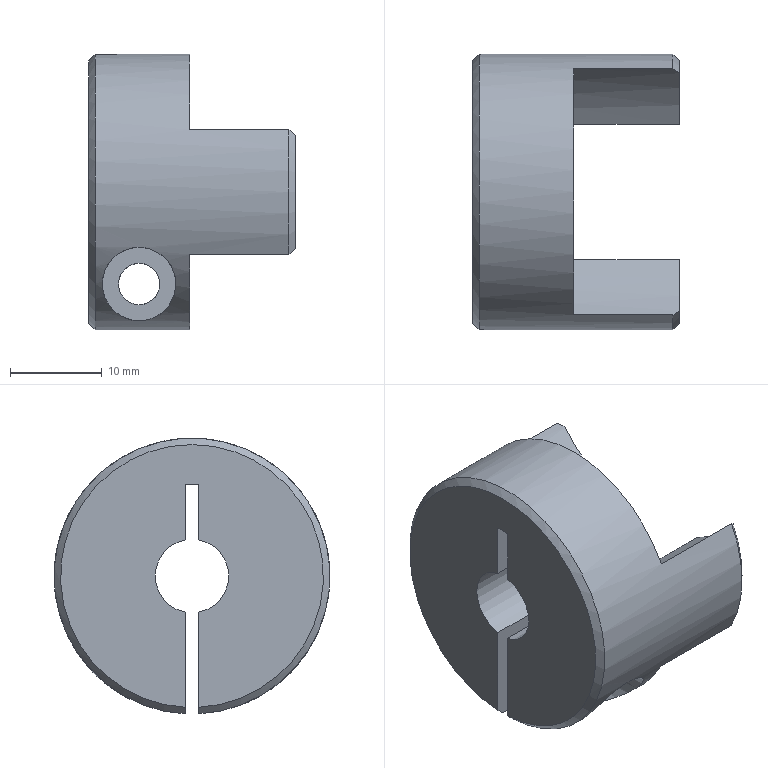Part | NX | features BREP 1 | 1 solid | 28 faces | box 22.5 x 30 x 29.981 mm | volume 7738 mm3 | cylinder 15 | plane 10 | cone 3 | commonest cylinder face diameters 4.5 x4 8 x4 32.5 x4 15 x2 30 x1
STEP:
#1=CARTESIAN_POINT('',(5.5,0.75,-12.25));
#2=VERTEX_POINT('',#1);
#3=CARTESIAN_POINT('',(5.5,0.75,-7.75));
#4=VERTEX_POINT('',#3);
#5=CARTESIAN_POINT('',(5.5,0.75,-10.));
#6=DIRECTION('',(0.,1.,0.));
#7=DIRECTION('',(0.,0.,1.));
#8=AXIS2_PLACEMENT_3D('',#5,#6,#7);
#9=CIRCLE('',#8,2.25);
#10=EDGE_CURVE('',#2,#4,#9,.T.);
#11=ORIENTED_EDGE('',*,*,#10,.F.);
#12=CARTESIAN_POINT('',(5.5,8.657,-12.25));
#13=VERTEX_POINT('',#12);
#14=CARTESIAN_POINT('',(5.5,13.748,-12.25));
#15=DIRECTION('',(0.,1.,0.));
#16=VECTOR('',#15,1000.);
#17=LINE('',#14,#16);
#18=EDGE_CURVE('',#2,#13,#17,.T.);
#19=ORIENTED_EDGE('',*,*,#18,.T.);
#20=CARTESIAN_POINT('',(5.5,12.843,-7.75));
#21=VERTEX_POINT('',#20);
#22=CARTESIAN_POINT('',(5.5,8.657,-12.25));
#23=CARTESIAN_POINT('',(4.786,8.657,-12.25));
#24=CARTESIAN_POINT('',(3.672,9.571,-11.603));
#25=CARTESIAN_POINT('',(3.097,11.052,-10.221));
#26=CARTESIAN_POINT('',(3.478,12.411,-8.494));
#27=CARTESIAN_POINT('',(4.788,12.843,-7.75));
#28=CARTESIAN_POINT('',(5.5,12.843,-7.75));
#29=B_SPLINE_CURVE_WITH_KNOTS('',3,(#22,#23,#24,#25,#26,#27,#28),.UNSPECIFIED.,.F.,.F.,(4,1,1,1,4),(0.,0.002109,0.004218,0.006326,0.008435),.UNSPECIFIED.);
#30=EDGE_CURVE('',#13,#21,#29,.T.);
#31=ORIENTED_EDGE('',*,*,#30,.T.);
#32=CARTESIAN_POINT('',(5.5,13.748,-7.75));
#33=DIRECTION('',(0.,1.,0.));
#34=VECTOR('',#33,1000.);
#35=LINE('',#32,#34);
#36=EDGE_CURVE('',#4,#21,#35,.T.);
#37=ORIENTED_EDGE('',*,*,#36,.F.);
#38=EDGE_LOOP('',(#11,#19,#31,#37));
#39=FACE_BOUND('',#38,.T.);
#40=CARTESIAN_POINT('',(5.5,13.748,-10.));
#41=DIRECTION('',(0.,1.,0.));
#42=DIRECTION('',(0.,0.,-1.));
#43=AXIS2_PLACEMENT_3D('',#40,#41,#42);
#44=CYLINDRICAL_SURFACE('',#43,2.25);
#45=ADVANCED_FACE('',(#39),#44,.F.);
#46=CARTESIAN_POINT('',(5.5,-13.748,-6.));
#47=VERTEX_POINT('',#46);
#48=CARTESIAN_POINT('',(5.5,-5.385,-14.));
#49=VERTEX_POINT('',#48);
#50=CARTESIAN_POINT('',(5.5,-13.748,-6.));
#51=CARTESIAN_POINT('',(4.181,-13.748,-6.));
#52=CARTESIAN_POINT('',(2.328,-13.314,-7.082));
#53=CARTESIAN_POINT('',(1.48,-11.906,-9.196));
#54=CARTESIAN_POINT('',(1.476,-10.6,-10.673));
#55=CARTESIAN_POINT('',(1.92,-9.153,-11.932));
#56=CARTESIAN_POINT('',(2.686,-7.669,-12.929));
#57=CARTESIAN_POINT('',(3.738,-6.207,-13.686));
#58=CARTESIAN_POINT('',(4.838,-5.385,-14.));
#59=CARTESIAN_POINT('',(5.5,-5.385,-14.));
#60=B_SPLINE_CURVE_WITH_KNOTS('',3,(#50,#51,#52,#53,#54,#55,#56,#57,#58,#59),.UNSPECIFIED.,.F.,.F.,(4,1,1,1,1,1,1,4),(0.,0.003899,0.005849,0.007799,0.009748,0.0117,0.01365,0.0156),.UNSPECIFIED.);
#61=EDGE_CURVE('',#47,#49,#60,.T.);
#62=ORIENTED_EDGE('',*,*,#61,.T.);
#63=CARTESIAN_POINT('',(5.5,-4.75,-14.));
#64=VERTEX_POINT('',#63);
#65=CARTESIAN_POINT('',(5.5,13.748,-14.));
#66=DIRECTION('',(0.,1.,0.));
#67=VECTOR('',#66,1000.);
#68=LINE('',#65,#67);
#69=EDGE_CURVE('',#64,#49,#68,.F.);
#70=ORIENTED_EDGE('',*,*,#69,.F.);
#71=CARTESIAN_POINT('',(5.5,-4.75,-6.));
#72=VERTEX_POINT('',#71);
#73=CARTESIAN_POINT('',(5.5,-4.75,-10.));
#74=DIRECTION('',(0.,1.,0.));
#75=DIRECTION('',(0.,0.,1.));
#76=AXIS2_PLACEMENT_3D('',#73,#74,#75);
#77=CIRCLE('',#76,4.);
#78=EDGE_CURVE('',#64,#72,#77,.T.);
#79=ORIENTED_EDGE('',*,*,#78,.T.);
#80=CARTESIAN_POINT('',(5.5,13.748,-6.));
#81=DIRECTION('',(0.,1.,0.));
#82=VECTOR('',#81,1000.);
#83=LINE('',#80,#82);
#84=EDGE_CURVE('',#72,#47,#83,.F.);
#85=ORIENTED_EDGE('',*,*,#84,.T.);
#86=EDGE_LOOP('',(#62,#70,#79,#85));
#87=FACE_BOUND('',#86,.T.);
#88=CARTESIAN_POINT('',(5.5,13.748,-10.));
#89=DIRECTION('',(0.,1.,0.));
#90=DIRECTION('',(0.,0.,-1.));
#91=AXIS2_PLACEMENT_3D('',#88,#89,#90);
#92=CYLINDRICAL_SURFACE('',#91,4.);
#93=ADVANCED_FACE('',(#87),#92,.F.);
#94=CARTESIAN_POINT('',(5.5,-4.75,-12.25));
#95=VERTEX_POINT('',#94);
#96=CARTESIAN_POINT('',(5.5,-4.75,-7.75));
#97=VERTEX_POINT('',#96);
#98=CARTESIAN_POINT('',(5.5,-4.75,-10.));
#99=DIRECTION('',(0.,1.,0.));
#100=DIRECTION('',(0.,0.,1.));
#101=AXIS2_PLACEMENT_3D('',#98,#99,#100);
#102=CIRCLE('',#101,2.25);
#103=EDGE_CURVE('',#95,#97,#102,.T.);
#104=ORIENTED_EDGE('',*,*,#103,.F.);
#105=CARTESIAN_POINT('',(5.5,-0.75,-12.25));
#106=VERTEX_POINT('',#105);
#107=CARTESIAN_POINT('',(5.5,13.748,-12.25));
#108=DIRECTION('',(0.,1.,0.));
#109=VECTOR('',#108,1000.);
#110=LINE('',#107,#109);
#111=EDGE_CURVE('',#95,#106,#110,.T.);
#112=ORIENTED_EDGE('',*,*,#111,.T.);
#113=CARTESIAN_POINT('',(5.5,-0.75,-7.75));
#114=VERTEX_POINT('',#113);
#115=CARTESIAN_POINT('',(5.5,-0.75,-10.));
#116=DIRECTION('',(0.,-1.,0.));
#117=DIRECTION('',(0.,0.,-1.));
#118=AXIS2_PLACEMENT_3D('',#115,#116,#117);
#119=CIRCLE('',#118,2.25);
#120=EDGE_CURVE('',#114,#106,#119,.T.);
#121=ORIENTED_EDGE('',*,*,#120,.F.);
#122=CARTESIAN_POINT('',(5.5,13.748,-7.75));
#123=DIRECTION('',(0.,1.,0.));
#124=VECTOR('',#123,1000.);
#125=LINE('',#122,#124);
#126=EDGE_CURVE('',#97,#114,#125,.T.);
#127=ORIENTED_EDGE('',*,*,#126,.F.);
#128=EDGE_LOOP('',(#104,#112,#121,#127));
#129=FACE_BOUND('',#128,.T.);
#130=CARTESIAN_POINT('',(5.5,13.748,-10.));
#131=DIRECTION('',(0.,1.,0.));
#132=DIRECTION('',(0.,0.,-1.));
#133=AXIS2_PLACEMENT_3D('',#130,#131,#132);
#134=CYLINDRICAL_SURFACE('',#133,2.25);
#135=ADVANCED_FACE('',(#129),#134,.F.);
#136=ORIENTED_EDGE('',*,*,#120,.T.);
#137=CARTESIAN_POINT('',(5.5,-0.75,-10.));
#138=DIRECTION('',(0.,-1.,0.));
#139=DIRECTION('',(0.,0.,-1.));
#140=AXIS2_PLACEMENT_3D('',#137,#138,#139);
#141=CIRCLE('',#140,2.25);
#142=EDGE_CURVE('',#106,#114,#141,.T.);
#143=ORIENTED_EDGE('',*,*,#142,.T.);
#144=EDGE_LOOP('',(#136,#143));
#145=FACE_BOUND('',#144,.T.);
#146=CARTESIAN_POINT('',(0.7071,-0.75,-14.981));
#147=VERTEX_POINT('',#146);
#148=CARTESIAN_POINT('',(11.,-0.75,-14.981));
#149=VERTEX_POINT('',#148);
#150=CARTESIAN_POINT('',(0.,-0.75,-14.981));
#151=DIRECTION('',(1.,0.,0.));
#152=VECTOR('',#151,1000.);
#153=LINE('',#150,#152);
#154=EDGE_CURVE('',#147,#149,#153,.T.);
#155=ORIENTED_EDGE('',*,*,#154,.F.);
#156=CARTESIAN_POINT('',(0.,-0.75,-14.273));
#157=VERTEX_POINT('',#156);
#158=CARTESIAN_POINT('',(0.7071,-0.75,-14.981));
#159=CARTESIAN_POINT('',(0.4714,-0.75,-14.745));
#160=CARTESIAN_POINT('',(0.2357,-0.75,-14.509));
#161=CARTESIAN_POINT('',(0.,-0.75,-14.273));
#162=B_SPLINE_CURVE_WITH_KNOTS('',3,(#158,#159,#160,#161),.UNSPECIFIED.,.F.,.F.,(4,4),(0.,1.),.PIECEWISE_BEZIER_KNOTS.);
#163=EDGE_CURVE('',#147,#157,#162,.T.);
#164=ORIENTED_EDGE('',*,*,#163,.T.);
#165=CARTESIAN_POINT('',(0.,-0.75,-3.929));
#166=VERTEX_POINT('',#165);
#167=CARTESIAN_POINT('',(0.,-0.75,10.));
#168=DIRECTION('',(0.,0.,-1.));
#169=VECTOR('',#168,1000.);
#170=LINE('',#167,#169);
#171=EDGE_CURVE('',#166,#157,#170,.T.);
#172=ORIENTED_EDGE('',*,*,#171,.F.);
#173=CARTESIAN_POINT('',(11.,-0.75,-3.929));
#174=VERTEX_POINT('',#173);
#175=CARTESIAN_POINT('',(0.,-0.75,-3.929));
#176=DIRECTION('',(1.,0.,0.));
#177=VECTOR('',#176,1000.);
#178=LINE('',#175,#177);
#179=EDGE_CURVE('',#166,#174,#178,.T.);
#180=ORIENTED_EDGE('',*,*,#179,.T.);
#181=CARTESIAN_POINT('',(11.,-0.75,10.));
#182=DIRECTION('',(0.,0.,-1.));
#183=VECTOR('',#182,1000.);
#184=LINE('',#181,#183);
#185=EDGE_CURVE('',#174,#149,#184,.T.);
#186=ORIENTED_EDGE('',*,*,#185,.T.);
#187=EDGE_LOOP('',(#155,#164,#172,#180,#186));
#188=FACE_BOUND('',#187,.T.);
#189=CARTESIAN_POINT('',(0.,-0.75,10.));
#190=DIRECTION('',(0.,-1.,0.));
#191=DIRECTION('',(0.,0.,1.));
#192=AXIS2_PLACEMENT_3D('',#189,#190,#191);
#193=PLANE('',#192);
#194=ADVANCED_FACE('',(#145,#188),#193,.F.);
#195=CARTESIAN_POINT('',(0.,0.75,3.929));
#196=VERTEX_POINT('',#195);
#197=CARTESIAN_POINT('',(0.,0.75,10.));
#198=VERTEX_POINT('',#197);
#199=CARTESIAN_POINT('',(0.,0.75,-14.981));
#200=DIRECTION('',(0.,0.,1.));
#201=VECTOR('',#200,1000.);
#202=LINE('',#199,#201);
#203=EDGE_CURVE('',#196,#198,#202,.T.);
#204=ORIENTED_EDGE('',*,*,#203,.F.);
#205=CARTESIAN_POINT('',(11.,0.75,3.929));
#206=VERTEX_POINT('',#205);
#207=CARTESIAN_POINT('',(0.,0.75,3.929));
#208=DIRECTION('',(1.,0.,0.));
#209=VECTOR('',#208,1000.);
#210=LINE('',#207,#209);
#211=EDGE_CURVE('',#196,#206,#210,.T.);
#212=ORIENTED_EDGE('',*,*,#211,.T.);
#213=CARTESIAN_POINT('',(11.,0.75,10.));
#214=VERTEX_POINT('',#213);
#215=CARTESIAN_POINT('',(11.,0.75,-14.981));
#216=DIRECTION('',(0.,0.,1.));
#217=VECTOR('',#216,1000.);
#218=LINE('',#215,#217);
#219=EDGE_CURVE('',#206,#214,#218,.T.);
#220=ORIENTED_EDGE('',*,*,#219,.T.);
#221=CARTESIAN_POINT('',(0.,0.75,10.));
#222=DIRECTION('',(1.,0.,0.));
#223=VECTOR('',#222,1000.);
#224=LINE('',#221,#223);
#225=EDGE_CURVE('',#198,#214,#224,.T.);
#226=ORIENTED_EDGE('',*,*,#225,.F.);
#227=EDGE_LOOP('',(#204,#212,#220,#226));
#228=FACE_BOUND('',#227,.T.);
#229=CARTESIAN_POINT('',(0.,0.75,-14.981));
#230=DIRECTION('',(0.,1.,0.));
#231=DIRECTION('',(0.,0.,-1.));
#232=AXIS2_PLACEMENT_3D('',#229,#230,#231);
#233=PLANE('',#232);
#234=ADVANCED_FACE('',(#228),#233,.F.);
#235=CARTESIAN_POINT('',(11.,-0.75,3.929));
#236=VERTEX_POINT('',#235);
#237=CARTESIAN_POINT('',(11.,0.,0.));
#238=DIRECTION('',(1.,0.,0.));
#239=DIRECTION('',(0.,0.,-1.));
#240=AXIS2_PLACEMENT_3D('',#237,#238,#239);
#241=CIRCLE('',#240,4.);
#242=EDGE_CURVE('',#236,#174,#241,.T.);
#243=ORIENTED_EDGE('',*,*,#242,.F.);
#244=CARTESIAN_POINT('',(11.,-0.75,10.));
#245=VERTEX_POINT('',#244);
#246=CARTESIAN_POINT('',(11.,-0.75,10.));
#247=DIRECTION('',(0.,0.,-1.));
#248=VECTOR('',#247,1000.);
#249=LINE('',#246,#248);
#250=EDGE_CURVE('',#245,#236,#249,.T.);
#251=ORIENTED_EDGE('',*,*,#250,.F.);
#252=CARTESIAN_POINT('',(11.,0.75,10.));
#253=DIRECTION('',(0.,-1.,0.));
#254=VECTOR('',#253,1000.);
#255=LINE('',#252,#254);
#256=EDGE_CURVE('',#214,#245,#255,.T.);
#257=ORIENTED_EDGE('',*,*,#256,.F.);
#258=ORIENTED_EDGE('',*,*,#219,.F.);
#259=CARTESIAN_POINT('',(11.,0.75,-3.929));
#260=VERTEX_POINT('',#259);
#261=CARTESIAN_POINT('',(11.,0.,0.));
#262=DIRECTION('',(1.,0.,0.));
#263=DIRECTION('',(0.,0.,-1.));
#264=AXIS2_PLACEMENT_3D('',#261,#262,#263);
#265=CIRCLE('',#264,4.);
#266=EDGE_CURVE('',#260,#206,#265,.T.);
#267=ORIENTED_EDGE('',*,*,#266,.F.);
#268=CARTESIAN_POINT('',(11.,0.75,-14.981));
#269=VERTEX_POINT('',#268);
#270=CARTESIAN_POINT('',(11.,0.75,-14.981));
#271=DIRECTION('',(0.,0.,1.));
#272=VECTOR('',#271,1000.);
#273=LINE('',#270,#272);
#274=EDGE_CURVE('',#269,#260,#273,.T.);
#275=ORIENTED_EDGE('',*,*,#274,.F.);
#276=CARTESIAN_POINT('',(11.,13.381,-6.779));
#277=VERTEX_POINT('',#276);
#278=CARTESIAN_POINT('',(11.,0.,0.));
#279=DIRECTION('',(1.,0.,0.));
#280=DIRECTION('',(0.,0.,-1.));
#281=AXIS2_PLACEMENT_3D('',#278,#279,#280);
#282=CIRCLE('',#281,15.);
#283=EDGE_CURVE('',#269,#277,#282,.T.);
#284=ORIENTED_EDGE('',*,*,#283,.T.);
#285=CARTESIAN_POINT('',(11.,7.347,-1.506));
#286=VERTEX_POINT('',#285);
#287=CARTESIAN_POINT('',(11.,0.,-16.));
#288=DIRECTION('',(-1.,0.,0.));
#289=DIRECTION('',(0.,0.,-1.));
#290=AXIS2_PLACEMENT_3D('',#287,#288,#289);
#291=CIRCLE('',#290,16.25);
#292=EDGE_CURVE('',#286,#277,#291,.T.);
#293=ORIENTED_EDGE('',*,*,#292,.F.);
#294=CARTESIAN_POINT('',(11.,7.347,1.506));
#295=VERTEX_POINT('',#294);
#296=CARTESIAN_POINT('',(11.,0.,0.));
#297=DIRECTION('',(-1.,0.,0.));
#298=DIRECTION('',(0.,0.,-1.));
#299=AXIS2_PLACEMENT_3D('',#296,#297,#298);
#300=CIRCLE('',#299,7.5);
#301=EDGE_CURVE('',#295,#286,#300,.T.);
#302=ORIENTED_EDGE('',*,*,#301,.F.);
#303=CARTESIAN_POINT('',(11.,13.381,6.779));
#304=VERTEX_POINT('',#303);
#305=CARTESIAN_POINT('',(11.,0.,16.));
#306=DIRECTION('',(-1.,0.,0.));
#307=DIRECTION('',(0.,0.,-1.));
#308=AXIS2_PLACEMENT_3D('',#305,#306,#307);
#309=CIRCLE('',#308,16.25);
#310=EDGE_CURVE('',#304,#295,#309,.T.);
#311=ORIENTED_EDGE('',*,*,#310,.F.);
#312=CARTESIAN_POINT('',(11.,-13.381,6.779));
#313=VERTEX_POINT('',#312);
#314=CARTESIAN_POINT('',(11.,0.,0.));
#315=DIRECTION('',(1.,0.,0.));
#316=DIRECTION('',(0.,0.,-1.));
#317=AXIS2_PLACEMENT_3D('',#314,#315,#316);
#318=CIRCLE('',#317,15.);
#319=EDGE_CURVE('',#304,#313,#318,.T.);
#320=ORIENTED_EDGE('',*,*,#319,.T.);
#321=CARTESIAN_POINT('',(11.,-7.347,1.506));
#322=VERTEX_POINT('',#321);
#323=CARTESIAN_POINT('',(11.,0.,16.));
#324=DIRECTION('',(1.,0.,0.));
#325=DIRECTION('',(0.,0.,-1.));
#326=AXIS2_PLACEMENT_3D('',#323,#324,#325);
#327=CIRCLE('',#326,16.25);
#328=EDGE_CURVE('',#313,#322,#327,.T.);
#329=ORIENTED_EDGE('',*,*,#328,.T.);
#330=CARTESIAN_POINT('',(11.,-7.347,-1.506));
#331=VERTEX_POINT('',#330);
#332=CARTESIAN_POINT('',(11.,0.,0.));
#333=DIRECTION('',(1.,0.,0.));
#334=DIRECTION('',(0.,0.,-1.));
#335=AXIS2_PLACEMENT_3D('',#332,#333,#334);
#336=CIRCLE('',#335,7.5);
#337=EDGE_CURVE('',#322,#331,#336,.T.);
#338=ORIENTED_EDGE('',*,*,#337,.T.);
#339=CARTESIAN_POINT('',(11.,-13.381,-6.779));
#340=VERTEX_POINT('',#339);
#341=CARTESIAN_POINT('',(11.,0.,-16.));
#342=DIRECTION('',(1.,0.,0.));
#343=DIRECTION('',(0.,0.,-1.));
#344=AXIS2_PLACEMENT_3D('',#341,#342,#343);
#345=CIRCLE('',#344,16.25);
#346=EDGE_CURVE('',#331,#340,#345,.T.);
#347=ORIENTED_EDGE('',*,*,#346,.T.);
#348=CARTESIAN_POINT('',(11.,0.,0.));
#349=DIRECTION('',(1.,0.,0.));
#350=DIRECTION('',(0.,0.,-1.));
#351=AXIS2_PLACEMENT_3D('',#348,#349,#350);
#352=CIRCLE('',#351,15.);
#353=EDGE_CURVE('',#340,#149,#352,.T.);
#354=ORIENTED_EDGE('',*,*,#353,.T.);
#355=ORIENTED_EDGE('',*,*,#185,.F.);
#356=EDGE_LOOP('',(#243,#251,#257,#258,#267,#275,#284,#293,#302,#311,#320,#329,#338,#347,#354,#355));
#357=FACE_BOUND('',#356,.T.);
#358=CARTESIAN_POINT('',(11.,0.,8.));
#359=DIRECTION('',(1.,0.,0.));
#360=DIRECTION('',(0.,0.,1.));
#361=AXIS2_PLACEMENT_3D('',#358,#359,#360);
#362=PLANE('',#361);
#363=ADVANCED_FACE('',(#357),#362,.T.);
#364=CARTESIAN_POINT('',(5.5,12.843,-7.75));
#365=CARTESIAN_POINT('',(6.211,12.843,-7.75));
#366=CARTESIAN_POINT('',(7.521,12.413,-8.492));
#367=CARTESIAN_POINT('',(7.904,11.052,-10.221));
#368=CARTESIAN_POINT('',(7.328,9.571,-11.603));
#369=CARTESIAN_POINT('',(6.214,8.657,-12.25));
#370=CARTESIAN_POINT('',(5.5,8.657,-12.25));
#371=B_SPLINE_CURVE_WITH_KNOTS('',3,(#364,#365,#366,#367,#368,#369,#370),.UNSPECIFIED.,.F.,.F.,(4,1,1,1,4),(0.,0.0021,0.004201,0.006301,0.008402),.UNSPECIFIED.);
#372=EDGE_CURVE('',#21,#13,#371,.T.);
#373=ORIENTED_EDGE('',*,*,#372,.F.);
#374=ORIENTED_EDGE('',*,*,#30,.F.);
#375=EDGE_LOOP('',(#373,#374));
#376=FACE_BOUND('',#375,.T.);
#377=ORIENTED_EDGE('',*,*,#61,.F.);
#378=CARTESIAN_POINT('',(5.5,-5.385,-14.));
#379=CARTESIAN_POINT('',(6.165,-5.385,-14.));
#380=CARTESIAN_POINT('',(7.265,-6.212,-13.683));
#381=CARTESIAN_POINT('',(8.31,-7.662,-12.934));
#382=CARTESIAN_POINT('',(9.083,-9.162,-11.923));
#383=CARTESIAN_POINT('',(9.667,-11.064,-10.283));
#384=CARTESIAN_POINT('',(9.299,-13.162,-7.484));
#385=CARTESIAN_POINT('',(6.823,-13.748,-6.));
#386=CARTESIAN_POINT('',(5.5,-13.748,-6.));
#387=B_SPLINE_CURVE_WITH_KNOTS('',3,(#378,#379,#380,#381,#382,#383,#384,#385,#386),.UNSPECIFIED.,.F.,.F.,(4,1,1,1,1,1,4),(0.,0.001957,0.003915,0.005872,0.00783,0.01174,0.01566),.UNSPECIFIED.);
#388=EDGE_CURVE('',#49,#47,#387,.T.);
#389=ORIENTED_EDGE('',*,*,#388,.F.);
#390=EDGE_LOOP('',(#377,#389));
#391=FACE_BOUND('',#390,.T.);
#392=CARTESIAN_POINT('',(21.793,-13.381,-6.779));
#393=VERTEX_POINT('',#392);
#394=CARTESIAN_POINT('',(11.,-13.381,-6.779));
#395=DIRECTION('',(1.,0.,0.));
#396=VECTOR('',#395,1000.);
#397=LINE('',#394,#396);
#398=EDGE_CURVE('',#340,#393,#397,.T.);
#399=ORIENTED_EDGE('',*,*,#398,.T.);
#400=CARTESIAN_POINT('',(21.793,-13.381,6.779));
#401=VERTEX_POINT('',#400);
#402=CARTESIAN_POINT('',(21.793,0.,0.));
#403=DIRECTION('',(-1.,0.,0.));
#404=DIRECTION('',(0.,0.,-1.));
#405=AXIS2_PLACEMENT_3D('',#402,#403,#404);
#406=CIRCLE('',#405,15.);
#407=EDGE_CURVE('',#393,#401,#406,.T.);
#408=ORIENTED_EDGE('',*,*,#407,.T.);
#409=CARTESIAN_POINT('',(11.,-13.381,6.779));
#410=DIRECTION('',(1.,0.,0.));
#411=VECTOR('',#410,1000.);
#412=LINE('',#409,#411);
#413=EDGE_CURVE('',#313,#401,#412,.T.);
#414=ORIENTED_EDGE('',*,*,#413,.F.);
#415=ORIENTED_EDGE('',*,*,#319,.F.);
#416=CARTESIAN_POINT('',(21.793,13.381,6.779));
#417=VERTEX_POINT('',#416);
#418=CARTESIAN_POINT('',(22.5,13.381,6.779));
#419=DIRECTION('',(-1.,0.,0.));
#420=VECTOR('',#419,1000.);
#421=LINE('',#418,#420);
#422=EDGE_CURVE('',#417,#304,#421,.T.);
#423=ORIENTED_EDGE('',*,*,#422,.F.);
#424=CARTESIAN_POINT('',(21.793,13.381,-6.779));
#425=VERTEX_POINT('',#424);
#426=CARTESIAN_POINT('',(21.793,0.,0.));
#427=DIRECTION('',(-1.,0.,0.));
#428=DIRECTION('',(0.,0.,-1.));
#429=AXIS2_PLACEMENT_3D('',#426,#427,#428);
#430=CIRCLE('',#429,15.);
#431=EDGE_CURVE('',#417,#425,#430,.T.);
#432=ORIENTED_EDGE('',*,*,#431,.T.);
#433=CARTESIAN_POINT('',(22.5,13.381,-6.779));
#434=DIRECTION('',(-1.,0.,0.));
#435=VECTOR('',#434,1000.);
#436=LINE('',#433,#435);
#437=EDGE_CURVE('',#425,#277,#436,.T.);
#438=ORIENTED_EDGE('',*,*,#437,.T.);
#439=ORIENTED_EDGE('',*,*,#283,.F.);
#440=CARTESIAN_POINT('',(0.7071,0.75,-14.981));
#441=VERTEX_POINT('',#440);
#442=CARTESIAN_POINT('',(0.,0.75,-14.981));
#443=DIRECTION('',(1.,0.,0.));
#444=VECTOR('',#443,1000.);
#445=LINE('',#442,#444);
#446=EDGE_CURVE('',#441,#269,#445,.T.);
#447=ORIENTED_EDGE('',*,*,#446,.F.);
#448=CARTESIAN_POINT('',(0.7071,0.,0.));
#449=DIRECTION('',(1.,0.,0.));
#450=DIRECTION('',(0.,0.,1.));
#451=AXIS2_PLACEMENT_3D('',#448,#449,#450);
#452=CIRCLE('',#451,15.);
#453=EDGE_CURVE('',#441,#147,#452,.T.);
#454=ORIENTED_EDGE('',*,*,#453,.T.);
#455=ORIENTED_EDGE('',*,*,#154,.T.);
#456=ORIENTED_EDGE('',*,*,#353,.F.);
#457=EDGE_LOOP('',(#399,#408,#414,#415,#423,#432,#438,#439,#447,#454,#455,#456));
#458=FACE_BOUND('',#457,.T.);
#459=CARTESIAN_POINT('',(0.,0.,0.));
#460=DIRECTION('',(1.,0.,0.));
#461=DIRECTION('',(0.,0.,1.));
#462=AXIS2_PLACEMENT_3D('',#459,#460,#461);
#463=CYLINDRICAL_SURFACE('',#462,15.);
#464=ADVANCED_FACE('',(#376,#391,#458),#463,.T.);
#465=ORIENTED_EDGE('',*,*,#171,.T.);
#466=CARTESIAN_POINT('',(0.,0.75,-14.273));
#467=VERTEX_POINT('',#466);
#468=CARTESIAN_POINT('',(0.,0.,0.));
#469=DIRECTION('',(-1.,0.,0.));
#470=DIRECTION('',(0.,0.,1.));
#471=AXIS2_PLACEMENT_3D('',#468,#469,#470);
#472=CIRCLE('',#471,14.293);
#473=EDGE_CURVE('',#157,#467,#472,.T.);
#474=ORIENTED_EDGE('',*,*,#473,.T.);
#475=CARTESIAN_POINT('',(0.,0.75,-3.929));
#476=VERTEX_POINT('',#475);
#477=CARTESIAN_POINT('',(0.,0.75,-14.981));
#478=DIRECTION('',(0.,0.,1.));
#479=VECTOR('',#478,1000.);
#480=LINE('',#477,#479);
#481=EDGE_CURVE('',#467,#476,#480,.T.);
#482=ORIENTED_EDGE('',*,*,#481,.T.);
#483=CARTESIAN_POINT('',(0.,0.,0.));
#484=DIRECTION('',(1.,0.,0.));
#485=DIRECTION('',(0.,0.,-1.));
#486=AXIS2_PLACEMENT_3D('',#483,#484,#485);
#487=CIRCLE('',#486,4.);
#488=EDGE_CURVE('',#476,#196,#487,.T.);
#489=ORIENTED_EDGE('',*,*,#488,.T.);
#490=ORIENTED_EDGE('',*,*,#203,.T.);
#491=CARTESIAN_POINT('',(0.,-0.75,10.));
#492=VERTEX_POINT('',#491);
#493=CARTESIAN_POINT('',(0.,0.75,10.));
#494=DIRECTION('',(0.,-1.,0.));
#495=VECTOR('',#494,1000.);
#496=LINE('',#493,#495);
#497=EDGE_CURVE('',#198,#492,#496,.T.);
#498=ORIENTED_EDGE('',*,*,#497,.T.);
#499=CARTESIAN_POINT('',(0.,-0.75,3.929));
#500=VERTEX_POINT('',#499);
#501=CARTESIAN_POINT('',(0.,-0.75,10.));
#502=DIRECTION('',(0.,0.,-1.));
#503=VECTOR('',#502,1000.);
#504=LINE('',#501,#503);
#505=EDGE_CURVE('',#492,#500,#504,.T.);
#506=ORIENTED_EDGE('',*,*,#505,.T.);
#507=CARTESIAN_POINT('',(0.,0.,0.));
#508=DIRECTION('',(1.,0.,0.));
#509=DIRECTION('',(0.,0.,-1.));
#510=AXIS2_PLACEMENT_3D('',#507,#508,#509);
#511=CIRCLE('',#510,4.);
#512=EDGE_CURVE('',#500,#166,#511,.T.);
#513=ORIENTED_EDGE('',*,*,#512,.T.);
#514=EDGE_LOOP('',(#465,#474,#482,#489,#490,#498,#506,#513));
#515=FACE_BOUND('',#514,.T.);
#516=CARTESIAN_POINT('',(0.,15.,0.));
#517=DIRECTION('',(-1.,0.,0.));
#518=DIRECTION('',(0.,0.,-1.));
#519=AXIS2_PLACEMENT_3D('',#516,#517,#518);
#520=PLANE('',#519);
#521=ADVANCED_FACE('',(#515),#520,.T.);
#522=CARTESIAN_POINT('',(22.5,-12.911,6.132));
#523=VERTEX_POINT('',#522);
#524=CARTESIAN_POINT('',(22.5,-7.347,1.506));
#525=VERTEX_POINT('',#524);
#526=CARTESIAN_POINT('',(22.5,0.,16.));
#527=DIRECTION('',(1.,0.,0.));
#528=DIRECTION('',(0.,0.,-1.));
#529=AXIS2_PLACEMENT_3D('',#526,#527,#528);
#530=CIRCLE('',#529,16.25);
#531=EDGE_CURVE('',#523,#525,#530,.T.);
#532=ORIENTED_EDGE('',*,*,#531,.F.);
#533=CARTESIAN_POINT('',(22.5,-12.911,-6.132));
#534=VERTEX_POINT('',#533);
#535=CARTESIAN_POINT('',(22.5,0.,0.));
#536=DIRECTION('',(1.,0.,0.));
#537=DIRECTION('',(0.,0.,-1.));
#538=AXIS2_PLACEMENT_3D('',#535,#536,#537);
#539=CIRCLE('',#538,14.293);
#540=EDGE_CURVE('',#523,#534,#539,.T.);
#541=ORIENTED_EDGE('',*,*,#540,.T.);
#542=CARTESIAN_POINT('',(22.5,-7.347,-1.506));
#543=VERTEX_POINT('',#542);
#544=CARTESIAN_POINT('',(22.5,0.,-16.));
#545=DIRECTION('',(1.,0.,0.));
#546=DIRECTION('',(0.,0.,-1.));
#547=AXIS2_PLACEMENT_3D('',#544,#545,#546);
#548=CIRCLE('',#547,16.25);
#549=EDGE_CURVE('',#543,#534,#548,.T.);
#550=ORIENTED_EDGE('',*,*,#549,.F.);
#551=CARTESIAN_POINT('',(22.5,0.,0.));
#552=DIRECTION('',(1.,0.,0.));
#553=DIRECTION('',(0.,0.,-1.));
#554=AXIS2_PLACEMENT_3D('',#551,#552,#553);
#555=CIRCLE('',#554,7.5);
#556=EDGE_CURVE('',#525,#543,#555,.T.);
#557=ORIENTED_EDGE('',*,*,#556,.F.);
#558=EDGE_LOOP('',(#532,#541,#550,#557));
#559=FACE_BOUND('',#558,.T.);
#560=CARTESIAN_POINT('',(22.5,0.,0.));
#561=DIRECTION('',(1.,0.,0.));
#562=DIRECTION('',(0.,0.,1.));
#563=AXIS2_PLACEMENT_3D('',#560,#561,#562);
#564=PLANE('',#563);
#565=ADVANCED_FACE('',(#559),#564,.T.);
#566=ORIENTED_EDGE('',*,*,#549,.T.);
#567=CARTESIAN_POINT('',(22.5,-12.911,-6.132));
#568=CARTESIAN_POINT('',(22.263,-13.072,-6.343));
#569=CARTESIAN_POINT('',(22.028,-13.229,-6.559));
#570=CARTESIAN_POINT('',(21.793,-13.381,-6.779));
#571=B_SPLINE_CURVE_WITH_KNOTS('',3,(#567,#568,#569,#570),.UNSPECIFIED.,.F.,.F.,(4,4),(0.,1.),.PIECEWISE_BEZIER_KNOTS.);
#572=EDGE_CURVE('',#534,#393,#571,.T.);
#573=ORIENTED_EDGE('',*,*,#572,.T.);
#574=ORIENTED_EDGE('',*,*,#398,.F.);
#575=ORIENTED_EDGE('',*,*,#346,.F.);
#576=CARTESIAN_POINT('',(11.,-7.347,-1.506));
#577=DIRECTION('',(1.,0.,0.));
#578=VECTOR('',#577,1000.);
#579=LINE('',#576,#578);
#580=EDGE_CURVE('',#331,#543,#579,.T.);
#581=ORIENTED_EDGE('',*,*,#580,.T.);
#582=EDGE_LOOP('',(#566,#573,#574,#575,#581));
#583=FACE_BOUND('',#582,.T.);
#584=CARTESIAN_POINT('',(11.,0.,-16.));
#585=DIRECTION('',(1.,0.,0.));
#586=DIRECTION('',(0.,0.,1.));
#587=AXIS2_PLACEMENT_3D('',#584,#585,#586);
#588=CYLINDRICAL_SURFACE('',#587,16.25);
#589=ADVANCED_FACE('',(#583),#588,.F.);
#590=ORIENTED_EDGE('',*,*,#556,.T.);
#591=ORIENTED_EDGE('',*,*,#580,.F.);
#592=ORIENTED_EDGE('',*,*,#337,.F.);
#593=CARTESIAN_POINT('',(11.,-7.347,1.506));
#594=DIRECTION('',(1.,0.,0.));
#595=VECTOR('',#594,1000.);
#596=LINE('',#593,#595);
#597=EDGE_CURVE('',#322,#525,#596,.T.);
#598=ORIENTED_EDGE('',*,*,#597,.T.);
#599=EDGE_LOOP('',(#590,#591,#592,#598));
#600=FACE_BOUND('',#599,.T.);
#601=CARTESIAN_POINT('',(11.,0.,0.));
#602=DIRECTION('',(1.,0.,0.));
#603=DIRECTION('',(0.,0.,1.));
#604=AXIS2_PLACEMENT_3D('',#601,#602,#603);
#605=CYLINDRICAL_SURFACE('',#604,7.5);
#606=ADVANCED_FACE('',(#600),#605,.F.);
#607=ORIENTED_EDGE('',*,*,#413,.T.);
#608=CARTESIAN_POINT('',(21.793,-13.381,6.779));
#609=CARTESIAN_POINT('',(22.028,-13.229,6.559));
#610=CARTESIAN_POINT('',(22.263,-13.072,6.343));
#611=CARTESIAN_POINT('',(22.5,-12.911,6.132));
#612=B_SPLINE_CURVE_WITH_KNOTS('',3,(#608,#609,#610,#611),.UNSPECIFIED.,.F.,.F.,(4,4),(0.,1.),.PIECEWISE_BEZIER_KNOTS.);
#613=EDGE_CURVE('',#401,#523,#612,.T.);
#614=ORIENTED_EDGE('',*,*,#613,.T.);
#615=ORIENTED_EDGE('',*,*,#531,.T.);
#616=ORIENTED_EDGE('',*,*,#597,.F.);
#617=ORIENTED_EDGE('',*,*,#328,.F.);
#618=EDGE_LOOP('',(#607,#614,#615,#616,#617));
#619=FACE_BOUND('',#618,.T.);
#620=CARTESIAN_POINT('',(11.,0.,16.));
#621=DIRECTION('',(1.,0.,0.));
#622=DIRECTION('',(0.,0.,1.));
#623=AXIS2_PLACEMENT_3D('',#620,#621,#622);
#624=CYLINDRICAL_SURFACE('',#623,16.25);
#625=ADVANCED_FACE('',(#619),#624,.F.);
#626=ORIENTED_EDGE('',*,*,#250,.T.);
#627=CARTESIAN_POINT('',(0.,-0.75,3.929));
#628=DIRECTION('',(1.,0.,0.));
#629=VECTOR('',#628,1000.);
#630=LINE('',#627,#629);
#631=EDGE_CURVE('',#500,#236,#630,.T.);
#632=ORIENTED_EDGE('',*,*,#631,.F.);
#633=ORIENTED_EDGE('',*,*,#505,.F.);
#634=CARTESIAN_POINT('',(0.,-0.75,10.));
#635=DIRECTION('',(1.,0.,0.));
#636=VECTOR('',#635,1000.);
#637=LINE('',#634,#636);
#638=EDGE_CURVE('',#492,#245,#637,.T.);
#639=ORIENTED_EDGE('',*,*,#638,.T.);
#640=EDGE_LOOP('',(#626,#632,#633,#639));
#641=FACE_BOUND('',#640,.T.);
#642=CARTESIAN_POINT('',(0.,-0.75,10.));
#643=DIRECTION('',(0.,-1.,0.));
#644=DIRECTION('',(0.,0.,1.));
#645=AXIS2_PLACEMENT_3D('',#642,#643,#644);
#646=PLANE('',#645);
#647=ADVANCED_FACE('',(#641),#646,.F.);
#648=ORIENTED_EDGE('',*,*,#256,.T.);
#649=ORIENTED_EDGE('',*,*,#638,.F.);
#650=ORIENTED_EDGE('',*,*,#497,.F.);
#651=ORIENTED_EDGE('',*,*,#225,.T.);
#652=EDGE_LOOP('',(#648,#649,#650,#651));
#653=FACE_BOUND('',#652,.T.);
#654=CARTESIAN_POINT('',(0.,0.75,10.));
#655=DIRECTION('',(0.,0.,1.));
#656=DIRECTION('',(-1.,0.,0.));
#657=AXIS2_PLACEMENT_3D('',#654,#655,#656);
#658=PLANE('',#657);
#659=ADVANCED_FACE('',(#653),#658,.F.);
#660=CARTESIAN_POINT('',(5.5,0.75,-10.));
#661=DIRECTION('',(0.,1.,0.));
#662=DIRECTION('',(0.,0.,1.));
#663=AXIS2_PLACEMENT_3D('',#660,#661,#662);
#664=CIRCLE('',#663,2.25);
#665=EDGE_CURVE('',#4,#2,#664,.T.);
#666=ORIENTED_EDGE('',*,*,#665,.T.);
#667=ORIENTED_EDGE('',*,*,#10,.T.);
#668=EDGE_LOOP('',(#666,#667));
#669=FACE_BOUND('',#668,.T.);
#670=ORIENTED_EDGE('',*,*,#481,.F.);
#671=CARTESIAN_POINT('',(0.,0.75,-14.273));
#672=CARTESIAN_POINT('',(0.2357,0.75,-14.509));
#673=CARTESIAN_POINT('',(0.4714,0.75,-14.745));
#674=CARTESIAN_POINT('',(0.7071,0.75,-14.981));
#675=B_SPLINE_CURVE_WITH_KNOTS('',3,(#671,#672,#673,#674),.UNSPECIFIED.,.F.,.F.,(4,4),(0.,1.),.PIECEWISE_BEZIER_KNOTS.);
#676=EDGE_CURVE('',#467,#441,#675,.T.);
#677=ORIENTED_EDGE('',*,*,#676,.T.);
#678=ORIENTED_EDGE('',*,*,#446,.T.);
#679=ORIENTED_EDGE('',*,*,#274,.T.);
#680=CARTESIAN_POINT('',(0.,0.75,-3.929));
#681=DIRECTION('',(1.,0.,0.));
#682=VECTOR('',#681,1000.);
#683=LINE('',#680,#682);
#684=EDGE_CURVE('',#476,#260,#683,.T.);
#685=ORIENTED_EDGE('',*,*,#684,.F.);
#686=EDGE_LOOP('',(#670,#677,#678,#679,#685));
#687=FACE_BOUND('',#686,.T.);
#688=CARTESIAN_POINT('',(0.,0.75,-14.981));
#689=DIRECTION('',(0.,1.,0.));
#690=DIRECTION('',(0.,0.,-1.));
#691=AXIS2_PLACEMENT_3D('',#688,#689,#690);
#692=PLANE('',#691);
#693=ADVANCED_FACE('',(#669,#687),#692,.F.);
#694=ORIENTED_EDGE('',*,*,#437,.F.);
#695=CARTESIAN_POINT('',(22.5,12.911,-6.132));
#696=VERTEX_POINT('',#695);
#697=CARTESIAN_POINT('',(21.793,13.381,-6.779));
#698=CARTESIAN_POINT('',(22.028,13.229,-6.559));
#699=CARTESIAN_POINT('',(22.263,13.072,-6.343));
#700=CARTESIAN_POINT('',(22.5,12.911,-6.132));
#701=B_SPLINE_CURVE_WITH_KNOTS('',3,(#697,#698,#699,#700),.UNSPECIFIED.,.F.,.F.,(4,4),(0.,1.),.PIECEWISE_BEZIER_KNOTS.);
#702=EDGE_CURVE('',#425,#696,#701,.T.);
#703=ORIENTED_EDGE('',*,*,#702,.T.);
#704=CARTESIAN_POINT('',(22.5,7.347,-1.506));
#705=VERTEX_POINT('',#704);
#706=CARTESIAN_POINT('',(22.5,0.,-16.));
#707=DIRECTION('',(-1.,0.,0.));
#708=DIRECTION('',(0.,0.,-1.));
#709=AXIS2_PLACEMENT_3D('',#706,#707,#708);
#710=CIRCLE('',#709,16.25);
#711=EDGE_CURVE('',#705,#696,#710,.T.);
#712=ORIENTED_EDGE('',*,*,#711,.F.);
#713=CARTESIAN_POINT('',(22.5,7.347,-1.506));
#714=DIRECTION('',(-1.,0.,0.));
#715=VECTOR('',#714,1000.);
#716=LINE('',#713,#715);
#717=EDGE_CURVE('',#705,#286,#716,.T.);
#718=ORIENTED_EDGE('',*,*,#717,.T.);
#719=ORIENTED_EDGE('',*,*,#292,.T.);
#720=EDGE_LOOP('',(#694,#703,#712,#718,#719));
#721=FACE_BOUND('',#720,.T.);
#722=CARTESIAN_POINT('',(22.5,0.,-16.));
#723=DIRECTION('',(-1.,0.,0.));
#724=DIRECTION('',(0.,0.,-1.));
#725=AXIS2_PLACEMENT_3D('',#722,#723,#724);
#726=CYLINDRICAL_SURFACE('',#725,16.25);
#727=ADVANCED_FACE('',(#721),#726,.F.);
#728=CARTESIAN_POINT('',(22.5,12.911,6.132));
#729=VERTEX_POINT('',#728);
#730=CARTESIAN_POINT('',(22.5,7.347,1.506));
#731=VERTEX_POINT('',#730);
#732=CARTESIAN_POINT('',(22.5,0.,16.));
#733=DIRECTION('',(-1.,0.,0.));
#734=DIRECTION('',(0.,0.,-1.));
#735=AXIS2_PLACEMENT_3D('',#732,#733,#734);
#736=CIRCLE('',#735,16.25);
#737=EDGE_CURVE('',#729,#731,#736,.T.);
#738=ORIENTED_EDGE('',*,*,#737,.F.);
#739=CARTESIAN_POINT('',(22.5,12.911,6.132));
#740=CARTESIAN_POINT('',(22.263,13.072,6.343));
#741=CARTESIAN_POINT('',(22.028,13.229,6.559));
#742=CARTESIAN_POINT('',(21.793,13.381,6.779));
#743=B_SPLINE_CURVE_WITH_KNOTS('',3,(#739,#740,#741,#742),.UNSPECIFIED.,.F.,.F.,(4,4),(0.,1.),.PIECEWISE_BEZIER_KNOTS.);
#744=EDGE_CURVE('',#729,#417,#743,.T.);
#745=ORIENTED_EDGE('',*,*,#744,.T.);
#746=ORIENTED_EDGE('',*,*,#422,.T.);
#747=ORIENTED_EDGE('',*,*,#310,.T.);
#748=CARTESIAN_POINT('',(22.5,7.347,1.506));
#749=DIRECTION('',(-1.,0.,0.));
#750=VECTOR('',#749,1000.);
#751=LINE('',#748,#750);
#752=EDGE_CURVE('',#731,#295,#751,.T.);
#753=ORIENTED_EDGE('',*,*,#752,.F.);
#754=EDGE_LOOP('',(#738,#745,#746,#747,#753));
#755=FACE_BOUND('',#754,.T.);
#756=CARTESIAN_POINT('',(22.5,0.,16.));
#757=DIRECTION('',(-1.,0.,0.));
#758=DIRECTION('',(0.,0.,-1.));
#759=AXIS2_PLACEMENT_3D('',#756,#757,#758);
#760=CYLINDRICAL_SURFACE('',#759,16.25);
#761=ADVANCED_FACE('',(#755),#760,.F.);
#762=ORIENTED_EDGE('',*,*,#301,.T.);
#763=ORIENTED_EDGE('',*,*,#717,.F.);
#764=CARTESIAN_POINT('',(22.5,0.,0.));
#765=DIRECTION('',(-1.,0.,0.));
#766=DIRECTION('',(0.,0.,-1.));
#767=AXIS2_PLACEMENT_3D('',#764,#765,#766);
#768=CIRCLE('',#767,7.5);
#769=EDGE_CURVE('',#731,#705,#768,.T.);
#770=ORIENTED_EDGE('',*,*,#769,.F.);
#771=ORIENTED_EDGE('',*,*,#752,.T.);
#772=EDGE_LOOP('',(#762,#763,#770,#771));
#773=FACE_BOUND('',#772,.T.);
#774=CARTESIAN_POINT('',(22.5,0.,0.));
#775=DIRECTION('',(-1.,0.,0.));
#776=DIRECTION('',(0.,0.,-1.));
#777=AXIS2_PLACEMENT_3D('',#774,#775,#776);
#778=CYLINDRICAL_SURFACE('',#777,7.5);
#779=ADVANCED_FACE('',(#773),#778,.F.);
#780=ORIENTED_EDGE('',*,*,#711,.T.);
#781=CARTESIAN_POINT('',(22.5,0.,0.));
#782=DIRECTION('',(1.,0.,0.));
#783=DIRECTION('',(0.,0.,-1.));
#784=AXIS2_PLACEMENT_3D('',#781,#782,#783);
#785=CIRCLE('',#784,14.293);
#786=EDGE_CURVE('',#696,#729,#785,.T.);
#787=ORIENTED_EDGE('',*,*,#786,.T.);
#788=ORIENTED_EDGE('',*,*,#737,.T.);
#789=ORIENTED_EDGE('',*,*,#769,.T.);
#790=EDGE_LOOP('',(#780,#787,#788,#789));
#791=FACE_BOUND('',#790,.T.);
#792=CARTESIAN_POINT('',(22.5,0.,-8.));
#793=DIRECTION('',(1.,0.,0.));
#794=DIRECTION('',(0.,0.,1.));
#795=AXIS2_PLACEMENT_3D('',#792,#793,#794);
#796=PLANE('',#795);
#797=ADVANCED_FACE('',(#791),#796,.T.);
#798=ORIENTED_EDGE('',*,*,#266,.T.);
#799=ORIENTED_EDGE('',*,*,#211,.F.);
#800=ORIENTED_EDGE('',*,*,#488,.F.);
#801=ORIENTED_EDGE('',*,*,#684,.T.);
#802=EDGE_LOOP('',(#798,#799,#800,#801));
#803=FACE_BOUND('',#802,.T.);
#804=CARTESIAN_POINT('',(0.,0.,0.));
#805=DIRECTION('',(1.,0.,0.));
#806=DIRECTION('',(0.,0.,1.));
#807=AXIS2_PLACEMENT_3D('',#804,#805,#806);
#808=CYLINDRICAL_SURFACE('',#807,4.);
#809=ADVANCED_FACE('',(#803),#808,.F.);
#810=ORIENTED_EDGE('',*,*,#242,.T.);
#811=ORIENTED_EDGE('',*,*,#179,.F.);
#812=ORIENTED_EDGE('',*,*,#512,.F.);
#813=ORIENTED_EDGE('',*,*,#631,.T.);
#814=EDGE_LOOP('',(#810,#811,#812,#813));
#815=FACE_BOUND('',#814,.T.);
#816=CARTESIAN_POINT('',(0.,0.,0.));
#817=DIRECTION('',(1.,0.,0.));
#818=DIRECTION('',(0.,0.,1.));
#819=AXIS2_PLACEMENT_3D('',#816,#817,#818);
#820=CYLINDRICAL_SURFACE('',#819,4.);
#821=ADVANCED_FACE('',(#815),#820,.F.);
#822=ORIENTED_EDGE('',*,*,#111,.F.);
#823=CARTESIAN_POINT('',(5.5,-4.75,-10.));
#824=DIRECTION('',(0.,1.,0.));
#825=DIRECTION('',(0.,0.,1.));
#826=AXIS2_PLACEMENT_3D('',#823,#824,#825);
#827=CIRCLE('',#826,2.25);
#828=EDGE_CURVE('',#97,#95,#827,.T.);
#829=ORIENTED_EDGE('',*,*,#828,.F.);
#830=ORIENTED_EDGE('',*,*,#126,.T.);
#831=ORIENTED_EDGE('',*,*,#142,.F.);
#832=EDGE_LOOP('',(#822,#829,#830,#831));
#833=FACE_BOUND('',#832,.T.);
#834=CARTESIAN_POINT('',(5.5,13.748,-10.));
#835=DIRECTION('',(0.,1.,0.));
#836=DIRECTION('',(0.,0.,-1.));
#837=AXIS2_PLACEMENT_3D('',#834,#835,#836);
#838=CYLINDRICAL_SURFACE('',#837,2.25);
#839=ADVANCED_FACE('',(#833),#838,.F.);
#840=CARTESIAN_POINT('',(5.5,-4.75,-10.));
#841=DIRECTION('',(0.,1.,0.));
#842=DIRECTION('',(0.,0.,1.));
#843=AXIS2_PLACEMENT_3D('',#840,#841,#842);
#844=CIRCLE('',#843,4.);
#845=EDGE_CURVE('',#72,#64,#844,.T.);
#846=ORIENTED_EDGE('',*,*,#845,.F.);
#847=ORIENTED_EDGE('',*,*,#78,.F.);
#848=EDGE_LOOP('',(#846,#847));
#849=FACE_BOUND('',#848,.T.);
#850=ORIENTED_EDGE('',*,*,#828,.T.);
#851=ORIENTED_EDGE('',*,*,#103,.T.);
#852=EDGE_LOOP('',(#850,#851));
#853=FACE_BOUND('',#852,.T.);
#854=CARTESIAN_POINT('',(9.5,-4.75,-10.));
#855=DIRECTION('',(0.,1.,0.));
#856=DIRECTION('',(0.,0.,-1.));
#857=AXIS2_PLACEMENT_3D('',#854,#855,#856);
#858=PLANE('',#857);
#859=ADVANCED_FACE('',(#849,#853),#858,.F.);
#860=ORIENTED_EDGE('',*,*,#69,.T.);
#861=ORIENTED_EDGE('',*,*,#388,.T.);
#862=ORIENTED_EDGE('',*,*,#84,.F.);
#863=ORIENTED_EDGE('',*,*,#845,.T.);
#864=EDGE_LOOP('',(#860,#861,#862,#863));
#865=FACE_BOUND('',#864,.T.);
#866=CARTESIAN_POINT('',(5.5,13.748,-10.));
#867=DIRECTION('',(0.,1.,0.));
#868=DIRECTION('',(0.,0.,-1.));
#869=AXIS2_PLACEMENT_3D('',#866,#867,#868);
#870=CYLINDRICAL_SURFACE('',#869,4.);
#871=ADVANCED_FACE('',(#865),#870,.F.);
#872=ORIENTED_EDGE('',*,*,#18,.F.);
#873=ORIENTED_EDGE('',*,*,#665,.F.);
#874=ORIENTED_EDGE('',*,*,#36,.T.);
#875=ORIENTED_EDGE('',*,*,#372,.T.);
#876=EDGE_LOOP('',(#872,#873,#874,#875));
#877=FACE_BOUND('',#876,.T.);
#878=CARTESIAN_POINT('',(5.5,13.748,-10.));
#879=DIRECTION('',(0.,1.,0.));
#880=DIRECTION('',(0.,0.,-1.));
#881=AXIS2_PLACEMENT_3D('',#878,#879,#880);
#882=CYLINDRICAL_SURFACE('',#881,2.25);
#883=ADVANCED_FACE('',(#877),#882,.F.);
#884=ORIENTED_EDGE('',*,*,#613,.F.);
#885=ORIENTED_EDGE('',*,*,#407,.F.);
#886=ORIENTED_EDGE('',*,*,#572,.F.);
#887=ORIENTED_EDGE('',*,*,#540,.F.);
#888=EDGE_LOOP('',(#884,#885,#886,#887));
#889=FACE_BOUND('',#888,.T.);
#890=CARTESIAN_POINT('',(22.5,0.,0.));
#891=DIRECTION('',(-1.,0.,0.));
#892=DIRECTION('',(0.,0.,-1.));
#893=AXIS2_PLACEMENT_3D('',#890,#891,#892);
#894=CONICAL_SURFACE('',#893,14.293,0.7854);
#895=ADVANCED_FACE('',(#889),#894,.T.);
#896=ORIENTED_EDGE('',*,*,#676,.F.);
#897=ORIENTED_EDGE('',*,*,#473,.F.);
#898=ORIENTED_EDGE('',*,*,#163,.F.);
#899=ORIENTED_EDGE('',*,*,#453,.F.);
#900=EDGE_LOOP('',(#896,#897,#898,#899));
#901=FACE_BOUND('',#900,.T.);
#902=CARTESIAN_POINT('',(0.7071,0.,0.));
#903=DIRECTION('',(1.,0.,0.));
#904=DIRECTION('',(0.,0.,1.));
#905=AXIS2_PLACEMENT_3D('',#902,#903,#904);
#906=CONICAL_SURFACE('',#905,15.,0.7854);
#907=ADVANCED_FACE('',(#901),#906,.T.);
#908=ORIENTED_EDGE('',*,*,#702,.F.);
#909=ORIENTED_EDGE('',*,*,#431,.F.);
#910=ORIENTED_EDGE('',*,*,#744,.F.);
#911=ORIENTED_EDGE('',*,*,#786,.F.);
#912=EDGE_LOOP('',(#908,#909,#910,#911));
#913=FACE_BOUND('',#912,.T.);
#914=CARTESIAN_POINT('',(22.5,0.,0.));
#915=DIRECTION('',(-1.,0.,0.));
#916=DIRECTION('',(0.,0.,-1.));
#917=AXIS2_PLACEMENT_3D('',#914,#915,#916);
#918=CONICAL_SURFACE('',#917,14.293,0.7854);
#919=ADVANCED_FACE('',(#913),#918,.T.);
#920=CLOSED_SHELL('',(#45,#93,#135,#194,#234,#363,#464,#521,#565,#589,#606,#625,#647,#659,#693,#727,#761,#779,#797,#809,#821,#839,#859,#871,#883,#895,#907,#919));
#921=MANIFOLD_SOLID_BREP('',#920);
#922=(LENGTH_UNIT()NAMED_UNIT(*)SI_UNIT(.MILLI.,.METRE.));
#923=UNCERTAINTY_MEASURE_WITH_UNIT(LENGTH_MEASURE(0.0508),#922,'','');
#924=(NAMED_UNIT(*)PLANE_ANGLE_UNIT()SI_UNIT($,.RADIAN.));
#925=(NAMED_UNIT(*)SI_UNIT($,.STERADIAN.)SOLID_ANGLE_UNIT());
#926=(GEOMETRIC_REPRESENTATION_CONTEXT(3)GLOBAL_UNCERTAINTY_ASSIGNED_CONTEXT((#923))GLOBAL_UNIT_ASSIGNED_CONTEXT((#922,#924,#925))REPRESENTATION_CONTEXT('',''));
#927=ADVANCED_BREP_SHAPE_REPRESENTATION('',(#921),#926);